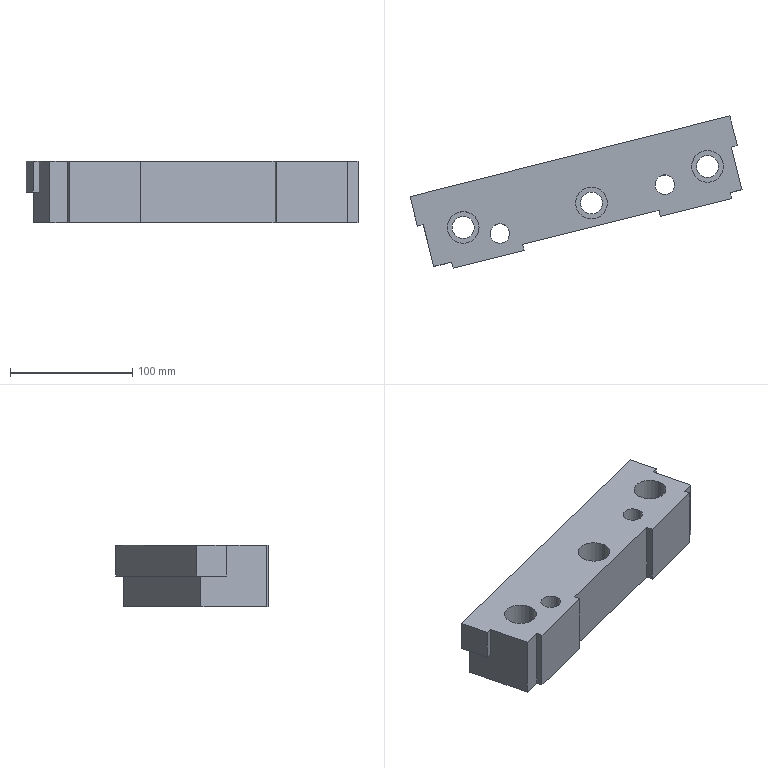Part | NX | features solid 2 | 1 solid | 31 faces | box 271.707 x 124.488 x 50 mm | volume 708876 mm3 | plane 19 | cylinder 8 | spline 4 | commonest cylinder face diameters 18 x3 26 x3 16 x2
STEP:
#1=CARTESIAN_POINT('',(-52.501,508.185,0.));
#2=VERTEX_POINT('',#1);
#3=CARTESIAN_POINT('',(-47.652,509.406,0.));
#4=VERTEX_POINT('',#3);
#5=CARTESIAN_POINT('',(-47.652,509.406,0.));
#6=CARTESIAN_POINT('',(-49.268,508.999,0.));
#7=CARTESIAN_POINT('',(-50.884,508.592,0.));
#8=CARTESIAN_POINT('',(-52.501,508.185,0.));
#9=B_SPLINE_CURVE_WITH_KNOTS('',3,(#5,#6,#7,#8),.UNSPECIFIED.,.F.,.F.,(4,4),(1.091,1.096),.UNSPECIFIED.);
#10=EDGE_CURVE('',#2,#4,#9,.F.);
#11=ORIENTED_EDGE('',*,*,#10,.F.);
#12=CARTESIAN_POINT('',(-52.501,508.185,-25.));
#13=VERTEX_POINT('',#12);
#14=CARTESIAN_POINT('',(-52.501,508.185,-25.));
#15=DIRECTION('',(0.,0.,-1.));
#16=VECTOR('',#15,1000.);
#17=LINE('',#14,#16);
#18=EDGE_CURVE('',#13,#2,#17,.F.);
#19=ORIENTED_EDGE('',*,*,#18,.F.);
#20=CARTESIAN_POINT('',(-47.652,509.406,-25.));
#21=VERTEX_POINT('',#20);
#22=CARTESIAN_POINT('',(-52.501,508.185,-25.));
#23=CARTESIAN_POINT('',(-50.884,508.592,-25.));
#24=CARTESIAN_POINT('',(-49.268,508.999,-25.));
#25=CARTESIAN_POINT('',(-47.652,509.406,-25.));
#26=B_SPLINE_CURVE_WITH_KNOTS('',3,(#22,#23,#24,#25),.UNSPECIFIED.,.F.,.F.,(4,4),(0.9813,0.9998),.UNSPECIFIED.);
#27=EDGE_CURVE('',#13,#21,#26,.T.);
#28=ORIENTED_EDGE('',*,*,#27,.T.);
#29=CARTESIAN_POINT('',(-47.652,509.406,-12.5));
#30=DIRECTION('',(0.,0.,-1.));
#31=VECTOR('',#30,1000.);
#32=LINE('',#29,#31);
#33=EDGE_CURVE('',#21,#4,#32,.F.);
#34=ORIENTED_EDGE('',*,*,#33,.T.);
#35=EDGE_LOOP('',(#11,#19,#28,#34));
#36=FACE_BOUND('',#35,.T.);
#37=CARTESIAN_POINT('',(-52.501,508.185,0.));
#38=CARTESIAN_POINT('',(-52.501,508.185,-25.));
#39=CARTESIAN_POINT('',(-50.884,508.592,0.));
#40=CARTESIAN_POINT('',(-50.884,508.592,-25.));
#41=CARTESIAN_POINT('',(-49.268,508.999,0.));
#42=CARTESIAN_POINT('',(-49.268,508.999,-25.));
#43=CARTESIAN_POINT('',(-47.652,509.406,0.));
#44=CARTESIAN_POINT('',(-47.652,509.406,-25.));
#45=B_SPLINE_SURFACE_WITH_KNOTS('',3,1,((#37,#38),(#39,#40),(#41,#42),(#43,#44)),.SURF_OF_LINEAR_EXTRUSION.,.F.,.F.,.F.,(4,4),(2,2),(0.9813,0.9998),(0.,1.),.PIECEWISE_BEZIER_KNOTS.);
#46=ADVANCED_FACE('',(#36),#45,.F.);
#47=CARTESIAN_POINT('',(-262.995,442.377,-50.));
#48=VERTEX_POINT('',#47);
#49=CARTESIAN_POINT('',(-271.995,442.377,-50.));
#50=DIRECTION('',(0.,0.,1.));
#51=DIRECTION('',(1.,0.,0.));
#52=AXIS2_PLACEMENT_3D('',#49,#50,#51);
#53=CIRCLE('',#52,9.);
#54=EDGE_CURVE('',#48,#48,#53,.T.);
#55=ORIENTED_EDGE('',*,*,#54,.F.);
#56=EDGE_LOOP('',(#55));
#57=FACE_BOUND('',#56,.T.);
#58=CARTESIAN_POINT('',(-262.995,442.377,-30.));
#59=VERTEX_POINT('',#58);
#60=CARTESIAN_POINT('',(-271.995,442.377,-30.));
#61=DIRECTION('',(0.,0.,1.));
#62=DIRECTION('',(1.,0.,0.));
#63=AXIS2_PLACEMENT_3D('',#60,#61,#62);
#64=CIRCLE('',#63,9.);
#65=EDGE_CURVE('',#59,#59,#64,.F.);
#66=ORIENTED_EDGE('',*,*,#65,.F.);
#67=EDGE_LOOP('',(#66));
#68=FACE_BOUND('',#67,.T.);
#69=CARTESIAN_POINT('',(-271.995,442.377,-125.));
#70=DIRECTION('',(0.,0.,1.));
#71=DIRECTION('',(1.,0.,0.));
#72=AXIS2_PLACEMENT_3D('',#69,#70,#71);
#73=CYLINDRICAL_SURFACE('',#72,9.);
#74=ADVANCED_FACE('',(#57,#68),#73,.F.);
#75=CARTESIAN_POINT('',(-157.995,462.377,-50.));
#76=VERTEX_POINT('',#75);
#77=CARTESIAN_POINT('',(-166.995,462.377,-50.));
#78=DIRECTION('',(0.,0.,1.));
#79=DIRECTION('',(1.,0.,0.));
#80=AXIS2_PLACEMENT_3D('',#77,#78,#79);
#81=CIRCLE('',#80,9.);
#82=EDGE_CURVE('',#76,#76,#81,.T.);
#83=ORIENTED_EDGE('',*,*,#82,.F.);
#84=EDGE_LOOP('',(#83));
#85=FACE_BOUND('',#84,.T.);
#86=CARTESIAN_POINT('',(-157.995,462.377,-30.));
#87=VERTEX_POINT('',#86);
#88=CARTESIAN_POINT('',(-166.995,462.377,-30.));
#89=DIRECTION('',(0.,0.,1.));
#90=DIRECTION('',(1.,0.,0.));
#91=AXIS2_PLACEMENT_3D('',#88,#89,#90);
#92=CIRCLE('',#91,9.);
#93=EDGE_CURVE('',#87,#87,#92,.F.);
#94=ORIENTED_EDGE('',*,*,#93,.F.);
#95=EDGE_LOOP('',(#94));
#96=FACE_BOUND('',#95,.T.);
#97=CARTESIAN_POINT('',(-166.995,462.377,-125.));
#98=DIRECTION('',(0.,0.,1.));
#99=DIRECTION('',(1.,0.,0.));
#100=AXIS2_PLACEMENT_3D('',#97,#98,#99);
#101=CYLINDRICAL_SURFACE('',#100,9.);
#102=ADVANCED_FACE('',(#85,#96),#101,.F.);
#103=CARTESIAN_POINT('',(-62.995,492.377,-50.));
#104=VERTEX_POINT('',#103);
#105=CARTESIAN_POINT('',(-71.995,492.377,-50.));
#106=DIRECTION('',(0.,0.,1.));
#107=DIRECTION('',(1.,0.,0.));
#108=AXIS2_PLACEMENT_3D('',#105,#106,#107);
#109=CIRCLE('',#108,9.);
#110=EDGE_CURVE('',#104,#104,#109,.T.);
#111=ORIENTED_EDGE('',*,*,#110,.F.);
#112=EDGE_LOOP('',(#111));
#113=FACE_BOUND('',#112,.T.);
#114=CARTESIAN_POINT('',(-62.995,492.377,-30.));
#115=VERTEX_POINT('',#114);
#116=CARTESIAN_POINT('',(-71.995,492.377,-30.));
#117=DIRECTION('',(0.,0.,1.));
#118=DIRECTION('',(1.,0.,0.));
#119=AXIS2_PLACEMENT_3D('',#116,#117,#118);
#120=CIRCLE('',#119,9.);
#121=EDGE_CURVE('',#115,#115,#120,.F.);
#122=ORIENTED_EDGE('',*,*,#121,.F.);
#123=EDGE_LOOP('',(#122));
#124=FACE_BOUND('',#123,.T.);
#125=CARTESIAN_POINT('',(-71.995,492.377,-125.));
#126=DIRECTION('',(0.,0.,1.));
#127=DIRECTION('',(1.,0.,0.));
#128=AXIS2_PLACEMENT_3D('',#125,#126,#127);
#129=CYLINDRICAL_SURFACE('',#128,9.);
#130=ADVANCED_FACE('',(#113,#124),#129,.F.);
#131=CARTESIAN_POINT('',(-43.802,473.297,0.));
#132=VERTEX_POINT('',#131);
#133=CARTESIAN_POINT('',(-53.505,470.878,0.));
#134=VERTEX_POINT('',#133);
#135=CARTESIAN_POINT('',(-300.93,409.188,0.));
#136=DIRECTION('',(-0.9703,-0.2419,0.));
#137=VECTOR('',#136,1000.);
#138=LINE('',#135,#137);
#139=EDGE_CURVE('',#132,#134,#138,.T.);
#140=ORIENTED_EDGE('',*,*,#139,.T.);
#141=CARTESIAN_POINT('',(-53.505,470.878,-50.));
#142=VERTEX_POINT('',#141);
#143=CARTESIAN_POINT('',(-53.505,470.878,-70.));
#144=DIRECTION('',(0.,0.,-1.));
#145=VECTOR('',#144,1000.);
#146=LINE('',#143,#145);
#147=EDGE_CURVE('',#134,#142,#146,.T.);
#148=ORIENTED_EDGE('',*,*,#147,.T.);
#149=CARTESIAN_POINT('',(-43.802,473.297,-50.));
#150=VERTEX_POINT('',#149);
#151=CARTESIAN_POINT('',(-363.329,393.63,-50.));
#152=DIRECTION('',(0.9703,0.2419,0.));
#153=VECTOR('',#152,1000.);
#154=LINE('',#151,#153);
#155=EDGE_CURVE('',#142,#150,#154,.T.);
#156=ORIENTED_EDGE('',*,*,#155,.T.);
#157=CARTESIAN_POINT('',(-43.802,473.297,-70.));
#158=DIRECTION('',(0.,0.,1.));
#159=VECTOR('',#158,1000.);
#160=LINE('',#157,#159);
#161=EDGE_CURVE('',#150,#132,#160,.T.);
#162=ORIENTED_EDGE('',*,*,#161,.T.);
#163=EDGE_LOOP('',(#140,#148,#156,#162));
#164=FACE_BOUND('',#163,.T.);
#165=CARTESIAN_POINT('',(-300.93,409.188,-70.));
#166=DIRECTION('',(0.2419,-0.9703,0.));
#167=DIRECTION('',(0.9703,0.2419,0.));
#168=AXIS2_PLACEMENT_3D('',#165,#166,#167);
#169=PLANE('',#168);
#170=ADVANCED_FACE('',(#164),#169,.T.);
#171=CARTESIAN_POINT('',(-111.723,456.363,0.));
#172=VERTEX_POINT('',#171);
#173=CARTESIAN_POINT('',(-111.723,456.363,-50.));
#174=VERTEX_POINT('',#173);
#175=CARTESIAN_POINT('',(-111.723,456.363,-70.));
#176=DIRECTION('',(0.,0.,-1.));
#177=VECTOR('',#176,1000.);
#178=LINE('',#175,#177);
#179=EDGE_CURVE('',#172,#174,#178,.T.);
#180=ORIENTED_EDGE('',*,*,#179,.F.);
#181=CARTESIAN_POINT('',(-223.307,428.542,0.));
#182=VERTEX_POINT('',#181);
#183=CARTESIAN_POINT('',(-300.93,409.188,0.));
#184=DIRECTION('',(-0.9703,-0.2419,0.));
#185=VECTOR('',#184,1000.);
#186=LINE('',#183,#185);
#187=EDGE_CURVE('',#172,#182,#186,.T.);
#188=ORIENTED_EDGE('',*,*,#187,.T.);
#189=CARTESIAN_POINT('',(-223.307,428.542,-50.));
#190=VERTEX_POINT('',#189);
#191=CARTESIAN_POINT('',(-223.307,428.542,-70.));
#192=DIRECTION('',(0.,0.,-1.));
#193=VECTOR('',#192,1000.);
#194=LINE('',#191,#193);
#195=EDGE_CURVE('',#182,#190,#194,.T.);
#196=ORIENTED_EDGE('',*,*,#195,.T.);
#197=CARTESIAN_POINT('',(-363.329,393.63,-50.));
#198=DIRECTION('',(0.9703,0.2419,0.));
#199=VECTOR('',#198,1000.);
#200=LINE('',#197,#199);
#201=EDGE_CURVE('',#190,#174,#200,.T.);
#202=ORIENTED_EDGE('',*,*,#201,.T.);
#203=EDGE_LOOP('',(#180,#188,#196,#202));
#204=FACE_BOUND('',#203,.T.);
#205=CARTESIAN_POINT('',(-300.93,409.188,-70.));
#206=DIRECTION('',(0.2419,-0.9703,0.));
#207=DIRECTION('',(0.9703,0.2419,0.));
#208=AXIS2_PLACEMENT_3D('',#205,#206,#207);
#209=PLANE('',#208);
#210=ADVANCED_FACE('',(#204),#209,.T.);
#211=CARTESIAN_POINT('',(-281.525,414.026,0.));
#212=VERTEX_POINT('',#211);
#213=CARTESIAN_POINT('',(-281.525,414.026,-50.));
#214=VERTEX_POINT('',#213);
#215=CARTESIAN_POINT('',(-281.525,414.026,-70.));
#216=DIRECTION('',(0.,0.,-1.));
#217=VECTOR('',#216,1000.);
#218=LINE('',#215,#217);
#219=EDGE_CURVE('',#212,#214,#218,.T.);
#220=ORIENTED_EDGE('',*,*,#219,.F.);
#221=CARTESIAN_POINT('',(-296.079,410.398,0.));
#222=VERTEX_POINT('',#221);
#223=CARTESIAN_POINT('',(-300.93,409.188,0.));
#224=DIRECTION('',(-0.9703,-0.2419,0.));
#225=VECTOR('',#224,1000.);
#226=LINE('',#223,#225);
#227=EDGE_CURVE('',#212,#222,#226,.T.);
#228=ORIENTED_EDGE('',*,*,#227,.T.);
#229=CARTESIAN_POINT('',(-296.079,410.398,-50.));
#230=VERTEX_POINT('',#229);
#231=CARTESIAN_POINT('',(-296.079,410.398,-70.));
#232=DIRECTION('',(0.,0.,1.));
#233=VECTOR('',#232,1000.);
#234=LINE('',#231,#233);
#235=EDGE_CURVE('',#230,#222,#234,.T.);
#236=ORIENTED_EDGE('',*,*,#235,.F.);
#237=CARTESIAN_POINT('',(-363.329,393.63,-50.));
#238=DIRECTION('',(0.9703,0.2419,0.));
#239=VECTOR('',#238,1000.);
#240=LINE('',#237,#239);
#241=EDGE_CURVE('',#230,#214,#240,.T.);
#242=ORIENTED_EDGE('',*,*,#241,.T.);
#243=EDGE_LOOP('',(#220,#228,#236,#242));
#244=FACE_BOUND('',#243,.T.);
#245=CARTESIAN_POINT('',(-300.93,409.188,-70.));
#246=DIRECTION('',(0.2419,-0.9703,0.));
#247=DIRECTION('',(0.9703,0.2419,0.));
#248=AXIS2_PLACEMENT_3D('',#245,#246,#247);
#249=PLANE('',#248);
#250=ADVANCED_FACE('',(#244),#249,.T.);
#251=CARTESIAN_POINT('',(-309.461,443.4,0.));
#252=VERTEX_POINT('',#251);
#253=CARTESIAN_POINT('',(-315.509,467.66,0.));
#254=VERTEX_POINT('',#253);
#255=CARTESIAN_POINT('',(14.033,-854.063,0.));
#256=DIRECTION('',(-0.2419,0.9703,0.));
#257=VECTOR('',#256,1000.);
#258=LINE('',#255,#257);
#259=EDGE_CURVE('',#252,#254,#258,.T.);
#260=ORIENTED_EDGE('',*,*,#259,.F.);
#261=CARTESIAN_POINT('',(-304.623,444.665,0.));
#262=VERTEX_POINT('',#261);
#263=CARTESIAN_POINT('',(-304.623,444.665,0.));
#264=CARTESIAN_POINT('',(-306.236,444.246,0.));
#265=CARTESIAN_POINT('',(-307.849,443.824,0.));
#266=CARTESIAN_POINT('',(-309.461,443.4,0.));
#267=B_SPLINE_CURVE_WITH_KNOTS('',3,(#263,#264,#265,#266),.UNSPECIFIED.,.F.,.F.,(4,4),(1.356,1.361),.UNSPECIFIED.);
#268=EDGE_CURVE('',#252,#262,#267,.F.);
#269=ORIENTED_EDGE('',*,*,#268,.T.);
#270=CARTESIAN_POINT('',(-285.193,366.734,0.));
#271=DIRECTION('',(0.2419,-0.9703,0.));
#272=VECTOR('',#271,1000.);
#273=LINE('',#270,#272);
#274=EDGE_CURVE('',#262,#222,#273,.T.);
#275=ORIENTED_EDGE('',*,*,#274,.T.);
#276=ORIENTED_EDGE('',*,*,#227,.F.);
#277=CARTESIAN_POINT('',(-280.315,409.175,0.));
#278=VERTEX_POINT('',#277);
#279=CARTESIAN_POINT('',(-296.103,472.498,0.));
#280=DIRECTION('',(0.2419,-0.9703,0.));
#281=VECTOR('',#280,1000.);
#282=LINE('',#279,#281);
#283=EDGE_CURVE('',#212,#278,#282,.T.);
#284=ORIENTED_EDGE('',*,*,#283,.T.);
#285=CARTESIAN_POINT('',(-222.097,423.69,0.));
#286=VERTEX_POINT('',#285);
#287=CARTESIAN_POINT('',(-362.119,388.779,0.));
#288=DIRECTION('',(0.9703,0.2419,0.));
#289=VECTOR('',#288,1000.);
#290=LINE('',#287,#289);
#291=EDGE_CURVE('',#278,#286,#290,.T.);
#292=ORIENTED_EDGE('',*,*,#291,.T.);
#293=CARTESIAN_POINT('',(-237.885,487.014,0.));
#294=DIRECTION('',(0.2419,-0.9703,0.));
#295=VECTOR('',#294,1000.);
#296=LINE('',#293,#295);
#297=EDGE_CURVE('',#182,#286,#296,.T.);
#298=ORIENTED_EDGE('',*,*,#297,.F.);
#299=ORIENTED_EDGE('',*,*,#187,.F.);
#300=CARTESIAN_POINT('',(-110.513,451.511,0.));
#301=VERTEX_POINT('',#300);
#302=CARTESIAN_POINT('',(-126.301,514.835,0.));
#303=DIRECTION('',(0.2419,-0.9703,0.));
#304=VECTOR('',#303,1000.);
#305=LINE('',#302,#304);
#306=EDGE_CURVE('',#172,#301,#305,.T.);
#307=ORIENTED_EDGE('',*,*,#306,.T.);
#308=CARTESIAN_POINT('',(-52.295,466.027,0.));
#309=VERTEX_POINT('',#308);
#310=CARTESIAN_POINT('',(-362.119,388.779,0.));
#311=DIRECTION('',(0.9703,0.2419,0.));
#312=VECTOR('',#311,1000.);
#313=LINE('',#310,#312);
#314=EDGE_CURVE('',#301,#309,#313,.T.);
#315=ORIENTED_EDGE('',*,*,#314,.T.);
#316=CARTESIAN_POINT('',(-68.084,529.35,0.));
#317=DIRECTION('',(0.2419,-0.9703,0.));
#318=VECTOR('',#317,1000.);
#319=LINE('',#316,#318);
#320=EDGE_CURVE('',#134,#309,#319,.T.);
#321=ORIENTED_EDGE('',*,*,#320,.F.);
#322=ORIENTED_EDGE('',*,*,#139,.F.);
#323=CARTESIAN_POINT('',(-32.916,429.634,0.));
#324=DIRECTION('',(0.2419,-0.9703,0.));
#325=VECTOR('',#324,1000.);
#326=LINE('',#323,#325);
#327=EDGE_CURVE('',#2,#132,#326,.T.);
#328=ORIENTED_EDGE('',*,*,#327,.F.);
#329=ORIENTED_EDGE('',*,*,#10,.T.);
#330=CARTESIAN_POINT('',(-53.7,533.663,0.));
#331=VERTEX_POINT('',#330);
#332=CARTESIAN_POINT('',(276.013,-788.744,0.));
#333=DIRECTION('',(-0.2419,0.9703,0.));
#334=VECTOR('',#333,1000.);
#335=LINE('',#332,#334);
#336=EDGE_CURVE('',#4,#331,#335,.T.);
#337=ORIENTED_EDGE('',*,*,#336,.T.);
#338=CARTESIAN_POINT('',(-53.7,533.663,0.));
#339=CARTESIAN_POINT('',(-75.519,528.17,0.));
#340=CARTESIAN_POINT('',(-119.156,517.175,0.));
#341=CARTESIAN_POINT('',(-184.597,500.638,0.));
#342=CARTESIAN_POINT('',(-239.173,486.991,0.));
#343=CARTESIAN_POINT('',(-282.82,476.03,0.));
#344=CARTESIAN_POINT('',(-304.634,470.521,0.));
#345=CARTESIAN_POINT('',(-315.509,467.66,0.));
#346=B_SPLINE_CURVE_WITH_KNOTS('',3,(#338,#339,#340,#341,#342,#343,#344,#345),.UNSPECIFIED.,.F.,.F.,(4,1,1,1,1,4),(2.049,2.116,2.184,2.251,2.285,2.319),.UNSPECIFIED.);
#347=EDGE_CURVE('',#254,#331,#346,.F.);
#348=ORIENTED_EDGE('',*,*,#347,.F.);
#349=EDGE_LOOP('',(#260,#269,#275,#276,#284,#292,#298,#299,#307,#315,#321,#322,#328,#329,#337,#348));
#350=FACE_BOUND('',#349,.T.);
#351=CARTESIAN_POINT('',(-258.995,442.377,0.));
#352=VERTEX_POINT('',#351);
#353=CARTESIAN_POINT('',(-271.995,442.377,0.));
#354=DIRECTION('',(0.,0.,1.));
#355=DIRECTION('',(1.,0.,0.));
#356=AXIS2_PLACEMENT_3D('',#353,#354,#355);
#357=CIRCLE('',#356,13.);
#358=EDGE_CURVE('',#352,#352,#357,.T.);
#359=ORIENTED_EDGE('',*,*,#358,.F.);
#360=EDGE_LOOP('',(#359));
#361=FACE_BOUND('',#360,.T.);
#362=CARTESIAN_POINT('',(-153.995,462.377,0.));
#363=VERTEX_POINT('',#362);
#364=CARTESIAN_POINT('',(-166.995,462.377,0.));
#365=DIRECTION('',(0.,0.,1.));
#366=DIRECTION('',(1.,0.,0.));
#367=AXIS2_PLACEMENT_3D('',#364,#365,#366);
#368=CIRCLE('',#367,13.);
#369=EDGE_CURVE('',#363,#363,#368,.T.);
#370=ORIENTED_EDGE('',*,*,#369,.F.);
#371=EDGE_LOOP('',(#370));
#372=FACE_BOUND('',#371,.T.);
#373=CARTESIAN_POINT('',(-58.995,492.377,0.));
#374=VERTEX_POINT('',#373);
#375=CARTESIAN_POINT('',(-71.995,492.377,0.));
#376=DIRECTION('',(0.,0.,1.));
#377=DIRECTION('',(1.,0.,0.));
#378=AXIS2_PLACEMENT_3D('',#375,#376,#377);
#379=CIRCLE('',#378,13.);
#380=EDGE_CURVE('',#374,#374,#379,.T.);
#381=ORIENTED_EDGE('',*,*,#380,.F.);
#382=EDGE_LOOP('',(#381));
#383=FACE_BOUND('',#382,.T.);
#384=CARTESIAN_POINT('',(-233.995,437.377,0.));
#385=VERTEX_POINT('',#384);
#386=CARTESIAN_POINT('',(-241.995,437.377,0.));
#387=DIRECTION('',(0.,0.,1.));
#388=DIRECTION('',(1.,0.,0.));
#389=AXIS2_PLACEMENT_3D('',#386,#387,#388);
#390=CIRCLE('',#389,8.);
#391=EDGE_CURVE('',#385,#385,#390,.T.);
#392=ORIENTED_EDGE('',*,*,#391,.F.);
#393=EDGE_LOOP('',(#392));
#394=FACE_BOUND('',#393,.T.);
#395=CARTESIAN_POINT('',(-98.995,477.377,0.));
#396=VERTEX_POINT('',#395);
#397=CARTESIAN_POINT('',(-106.995,477.377,0.));
#398=DIRECTION('',(0.,0.,1.));
#399=DIRECTION('',(1.,0.,0.));
#400=AXIS2_PLACEMENT_3D('',#397,#398,#399);
#401=CIRCLE('',#400,8.);
#402=EDGE_CURVE('',#396,#396,#401,.T.);
#403=ORIENTED_EDGE('',*,*,#402,.F.);
#404=EDGE_LOOP('',(#403));
#405=FACE_BOUND('',#404,.T.);
#406=CARTESIAN_POINT('',(-48.365,-869.621,0.));
#407=DIRECTION('',(0.,0.,1.));
#408=DIRECTION('',(1.,0.,0.));
#409=AXIS2_PLACEMENT_3D('',#406,#407,#408);
#410=PLANE('',#409);
#411=ADVANCED_FACE('',(#350,#361,#372,#383,#394,#405),#410,.T.);
#412=CARTESIAN_POINT('',(-309.461,443.4,-25.));
#413=VERTEX_POINT('',#412);
#414=CARTESIAN_POINT('',(-304.623,444.665,-25.));
#415=VERTEX_POINT('',#414);
#416=CARTESIAN_POINT('',(-309.461,443.4,-25.));
#417=CARTESIAN_POINT('',(-307.824,443.831,-25.));
#418=CARTESIAN_POINT('',(-306.238,444.246,-25.));
#419=CARTESIAN_POINT('',(-304.623,444.665,-25.));
#420=B_SPLINE_CURVE_WITH_KNOTS('',3,(#416,#417,#418,#419),.UNSPECIFIED.,.F.,.F.,(4,4),(-0.001195,0.01761),.UNSPECIFIED.);
#421=EDGE_CURVE('',#413,#415,#420,.T.);
#422=ORIENTED_EDGE('',*,*,#421,.F.);
#423=CARTESIAN_POINT('',(-315.509,467.66,-25.));
#424=VERTEX_POINT('',#423);
#425=CARTESIAN_POINT('',(-315.509,467.66,-25.));
#426=DIRECTION('',(0.2419,-0.9703,0.));
#427=VECTOR('',#426,1000.);
#428=LINE('',#425,#427);
#429=EDGE_CURVE('',#424,#413,#428,.T.);
#430=ORIENTED_EDGE('',*,*,#429,.F.);
#431=CARTESIAN_POINT('',(-53.7,533.663,-25.));
#432=VERTEX_POINT('',#431);
#433=CARTESIAN_POINT('',(-315.509,467.66,-25.));
#434=CARTESIAN_POINT('',(-304.633,470.521,-25.));
#435=CARTESIAN_POINT('',(-282.818,476.031,-25.));
#436=CARTESIAN_POINT('',(-239.172,486.991,-25.));
#437=CARTESIAN_POINT('',(-184.599,500.638,-25.));
#438=CARTESIAN_POINT('',(-119.156,517.175,-25.));
#439=CARTESIAN_POINT('',(-75.519,528.17,-25.));
#440=CARTESIAN_POINT('',(-53.7,533.663,-25.));
#441=B_SPLINE_CURVE_WITH_KNOTS('',3,(#433,#434,#435,#436,#437,#438,#439,#440),.UNSPECIFIED.,.F.,.F.,(4,1,1,1,1,4),(0.4881,0.5217,0.5553,0.6226,0.6898,0.757),.UNSPECIFIED.);
#442=EDGE_CURVE('',#424,#432,#441,.T.);
#443=ORIENTED_EDGE('',*,*,#442,.T.);
#444=CARTESIAN_POINT('',(558.557,-1921.963,-25.));
#445=DIRECTION('',(-0.2419,0.9703,0.));
#446=VECTOR('',#445,1000.);
#447=LINE('',#444,#446);
#448=EDGE_CURVE('',#21,#432,#447,.T.);
#449=ORIENTED_EDGE('',*,*,#448,.F.);
#450=ORIENTED_EDGE('',*,*,#27,.F.);
#451=CARTESIAN_POINT('',(-57.339,527.591,-25.));
#452=VERTEX_POINT('',#451);
#453=CARTESIAN_POINT('',(-32.916,429.634,-25.));
#454=DIRECTION('',(-0.2419,0.9703,0.));
#455=VECTOR('',#454,1000.);
#456=LINE('',#453,#455);
#457=EDGE_CURVE('',#13,#452,#456,.T.);
#458=ORIENTED_EDGE('',*,*,#457,.T.);
#459=CARTESIAN_POINT('',(-309.462,464.072,-25.));
#460=VERTEX_POINT('',#459);
#461=CARTESIAN_POINT('',(-57.339,527.591,-25.));
#462=CARTESIAN_POINT('',(-78.35,522.301,-25.));
#463=CARTESIAN_POINT('',(-120.369,511.708,-25.));
#464=CARTESIAN_POINT('',(-183.392,495.797,-25.));
#465=CARTESIAN_POINT('',(-246.439,479.985,-25.));
#466=CARTESIAN_POINT('',(-288.49,469.519,-25.));
#467=CARTESIAN_POINT('',(-309.462,464.072,-25.));
#468=B_SPLINE_CURVE_WITH_KNOTS('',3,(#461,#462,#463,#464,#465,#466,#467),.UNSPECIFIED.,.F.,.F.,(4,1,1,1,4),(1.096,1.161,1.226,1.291,1.356),.UNSPECIFIED.);
#469=EDGE_CURVE('',#460,#452,#468,.F.);
#470=ORIENTED_EDGE('',*,*,#469,.F.);
#471=CARTESIAN_POINT('',(-285.193,366.734,-25.));
#472=DIRECTION('',(-0.2419,0.9703,0.));
#473=VECTOR('',#472,1000.);
#474=LINE('',#471,#473);
#475=EDGE_CURVE('',#415,#460,#474,.T.);
#476=ORIENTED_EDGE('',*,*,#475,.F.);
#477=EDGE_LOOP('',(#422,#430,#443,#449,#450,#458,#470,#476));
#478=FACE_BOUND('',#477,.T.);
#479=CARTESIAN_POINT('',(-315.509,467.66,-25.));
#480=DIRECTION('',(0.,0.,-1.));
#481=DIRECTION('',(-1.,0.,0.));
#482=AXIS2_PLACEMENT_3D('',#479,#480,#481);
#483=PLANE('',#482);
#484=ADVANCED_FACE('',(#478),#483,.T.);
#485=ORIENTED_EDGE('',*,*,#457,.F.);
#486=ORIENTED_EDGE('',*,*,#18,.T.);
#487=ORIENTED_EDGE('',*,*,#327,.T.);
#488=ORIENTED_EDGE('',*,*,#161,.F.);
#489=CARTESIAN_POINT('',(-57.339,527.591,-50.));
#490=VERTEX_POINT('',#489);
#491=CARTESIAN_POINT('',(271.162,-789.954,-50.));
#492=DIRECTION('',(-0.2419,0.9703,0.));
#493=VECTOR('',#492,1000.);
#494=LINE('',#491,#493);
#495=EDGE_CURVE('',#150,#490,#494,.T.);
#496=ORIENTED_EDGE('',*,*,#495,.T.);
#497=CARTESIAN_POINT('',(-57.339,527.591,-42.5));
#498=DIRECTION('',(0.,0.,1.));
#499=VECTOR('',#498,1000.);
#500=LINE('',#497,#499);
#501=EDGE_CURVE('',#490,#452,#500,.T.);
#502=ORIENTED_EDGE('',*,*,#501,.T.);
#503=EDGE_LOOP('',(#485,#486,#487,#488,#496,#502));
#504=FACE_BOUND('',#503,.T.);
#505=CARTESIAN_POINT('',(-32.916,429.634,-70.));
#506=DIRECTION('',(0.9703,0.2419,0.));
#507=DIRECTION('',(-0.2419,0.9703,0.));
#508=AXIS2_PLACEMENT_3D('',#505,#506,#507);
#509=PLANE('',#508);
#510=ADVANCED_FACE('',(#504),#509,.T.);
#511=ORIENTED_EDGE('',*,*,#274,.F.);
#512=CARTESIAN_POINT('',(-304.623,444.665,-25.));
#513=DIRECTION('',(0.,0.,-1.));
#514=VECTOR('',#513,1000.);
#515=LINE('',#512,#514);
#516=EDGE_CURVE('',#415,#262,#515,.F.);
#517=ORIENTED_EDGE('',*,*,#516,.F.);
#518=ORIENTED_EDGE('',*,*,#475,.T.);
#519=CARTESIAN_POINT('',(-309.462,464.072,-50.));
#520=VERTEX_POINT('',#519);
#521=CARTESIAN_POINT('',(-309.462,464.072,-42.5));
#522=DIRECTION('',(0.,0.,1.));
#523=VECTOR('',#522,1000.);
#524=LINE('',#521,#523);
#525=EDGE_CURVE('',#520,#460,#524,.T.);
#526=ORIENTED_EDGE('',*,*,#525,.F.);
#527=CARTESIAN_POINT('',(18.885,-852.853,-50.));
#528=DIRECTION('',(-0.2419,0.9703,0.));
#529=VECTOR('',#528,1000.);
#530=LINE('',#527,#529);
#531=EDGE_CURVE('',#230,#520,#530,.T.);
#532=ORIENTED_EDGE('',*,*,#531,.F.);
#533=ORIENTED_EDGE('',*,*,#235,.T.);
#534=EDGE_LOOP('',(#511,#517,#518,#526,#532,#533));
#535=FACE_BOUND('',#534,.T.);
#536=CARTESIAN_POINT('',(-285.193,366.734,-70.));
#537=DIRECTION('',(0.9703,0.2419,0.));
#538=DIRECTION('',(-0.2419,0.9703,0.));
#539=AXIS2_PLACEMENT_3D('',#536,#537,#538);
#540=PLANE('',#539);
#541=ADVANCED_FACE('',(#535),#540,.F.);
#542=ORIENTED_EDGE('',*,*,#54,.T.);
#543=EDGE_LOOP('',(#542));
#544=FACE_BOUND('',#543,.T.);
#545=CARTESIAN_POINT('',(-233.995,437.377,-50.));
#546=VERTEX_POINT('',#545);
#547=CARTESIAN_POINT('',(-241.995,437.377,-50.));
#548=DIRECTION('',(0.,0.,1.));
#549=DIRECTION('',(1.,0.,0.));
#550=AXIS2_PLACEMENT_3D('',#547,#548,#549);
#551=CIRCLE('',#550,8.);
#552=EDGE_CURVE('',#546,#546,#551,.T.);
#553=ORIENTED_EDGE('',*,*,#552,.T.);
#554=EDGE_LOOP('',(#553));
#555=FACE_BOUND('',#554,.T.);
#556=ORIENTED_EDGE('',*,*,#82,.T.);
#557=EDGE_LOOP('',(#556));
#558=FACE_BOUND('',#557,.T.);
#559=CARTESIAN_POINT('',(-98.995,477.377,-50.));
#560=VERTEX_POINT('',#559);
#561=CARTESIAN_POINT('',(-106.995,477.377,-50.));
#562=DIRECTION('',(0.,0.,1.));
#563=DIRECTION('',(1.,0.,0.));
#564=AXIS2_PLACEMENT_3D('',#561,#562,#563);
#565=CIRCLE('',#564,8.);
#566=EDGE_CURVE('',#560,#560,#565,.T.);
#567=ORIENTED_EDGE('',*,*,#566,.T.);
#568=EDGE_LOOP('',(#567));
#569=FACE_BOUND('',#568,.T.);
#570=ORIENTED_EDGE('',*,*,#110,.T.);
#571=EDGE_LOOP('',(#570));
#572=FACE_BOUND('',#571,.T.);
#573=ORIENTED_EDGE('',*,*,#531,.T.);
#574=CARTESIAN_POINT('',(-309.462,464.072,-50.));
#575=CARTESIAN_POINT('',(-306.559,464.826,-50.));
#576=CARTESIAN_POINT('',(-301.325,466.172,-50.));
#577=CARTESIAN_POINT('',(-292.584,468.397,-50.));
#578=CARTESIAN_POINT('',(-285.148,470.281,-50.));
#579=CARTESIAN_POINT('',(-276.83,472.38,-50.));
#580=CARTESIAN_POINT('',(-269.164,474.308,-50.));
#581=CARTESIAN_POINT('',(-262.592,475.958,-50.));
#582=CARTESIAN_POINT('',(-257.439,477.251,-50.));
#583=CARTESIAN_POINT('',(-252.972,478.37,-50.));
#584=CARTESIAN_POINT('',(-249.729,479.182,-50.));
#585=CARTESIAN_POINT('',(-247.88,479.645,-50.));
#586=CARTESIAN_POINT('',(-246.389,480.018,-50.));
#587=CARTESIAN_POINT('',(-245.229,480.308,-50.));
#588=CARTESIAN_POINT('',(-243.58,480.72,-50.));
#589=CARTESIAN_POINT('',(-240.775,481.422,-50.));
#590=CARTESIAN_POINT('',(-236.816,482.413,-50.));
#591=CARTESIAN_POINT('',(-232.2,483.568,-50.));
#592=CARTESIAN_POINT('',(-226.206,485.069,-50.));
#593=CARTESIAN_POINT('',(-219.023,486.869,-50.));
#594=CARTESIAN_POINT('',(-210.895,488.906,-50.));
#595=CARTESIAN_POINT('',(-203.261,490.821,-50.));
#596=CARTESIAN_POINT('',(-197.309,492.315,-50.));
#597=CARTESIAN_POINT('',(-192.795,493.449,-50.));
#598=CARTESIAN_POINT('',(-189.529,494.27,-50.));
#599=CARTESIAN_POINT('',(-186.922,494.926,-50.));
#600=CARTESIAN_POINT('',(-185.128,495.377,-50.));
#601=CARTESIAN_POINT('',(-184.154,495.623,-50.));
#602=CARTESIAN_POINT('',(-183.332,495.829,-50.));
#603=CARTESIAN_POINT('',(-182.894,495.94,-50.));
#604=CARTESIAN_POINT('',(-182.151,496.127,-50.));
#605=CARTESIAN_POINT('',(-180.865,496.451,-50.));
#606=CARTESIAN_POINT('',(-178.846,496.959,-50.));
#607=CARTESIAN_POINT('',(-176.203,497.625,-50.));
#608=CARTESIAN_POINT('',(-172.36,498.593,-50.));
#609=CARTESIAN_POINT('',(-166.971,499.951,-50.));
#610=CARTESIAN_POINT('',(-159.563,501.819,-50.));
#611=CARTESIAN_POINT('',(-151.214,503.924,-50.));
#612=CARTESIAN_POINT('',(-143.473,505.876,-50.));
#613=CARTESIAN_POINT('',(-136.81,507.557,-50.));
#614=CARTESIAN_POINT('',(-132.449,508.657,-50.));
#615=CARTESIAN_POINT('',(-128.844,509.566,-50.));
#616=CARTESIAN_POINT('',(-126.078,510.264,-50.));
#617=CARTESIAN_POINT('',(-123.735,510.855,-50.));
#618=CARTESIAN_POINT('',(-122.048,511.281,-50.));
#619=CARTESIAN_POINT('',(-121.11,511.517,-50.));
#620=CARTESIAN_POINT('',(-120.31,511.719,-50.));
#621=CARTESIAN_POINT('',(-119.859,511.833,-50.));
#622=CARTESIAN_POINT('',(-119.138,512.015,-50.));
#623=CARTESIAN_POINT('',(-117.934,512.319,-50.));
#624=CARTESIAN_POINT('',(-116.189,512.759,-50.));
#625=CARTESIAN_POINT('',(-114.115,513.282,-50.));
#626=CARTESIAN_POINT('',(-111.357,513.978,-50.));
#627=CARTESIAN_POINT('',(-107.93,514.842,-50.));
#628=CARTESIAN_POINT('',(-102.488,516.214,-50.));
#629=CARTESIAN_POINT('',(-95.764,517.909,-50.));
#630=CARTESIAN_POINT('',(-87.823,519.911,-50.));
#631=CARTESIAN_POINT('',(-80.007,521.881,-50.));
#632=CARTESIAN_POINT('',(-69.755,524.464,-50.));
#633=CARTESIAN_POINT('',(-62.255,526.353,-50.));
#634=CARTESIAN_POINT('',(-57.339,527.591,-50.));
#635=B_SPLINE_CURVE_WITH_KNOTS('',3,(#574,#575,#576,#577,#578,#579,#580,#581,#582,#583,#584,#585,#586,#587,#588,#589,#590,#591,#592,#593,#594,#595,#596,#597,#598,#599,#600,#601,#602,#603,#604,#605,#606,#607,#608,#609,#610,#611,#612,#613,#614,#615,#616,#617,#618,#619,#620,#621,#622,#623,#624,#625,#626,#627,#628,#629,#630,#631,#632,#633,#634),.UNSPECIFIED.,.F.,.F.,(4,1,1,1,1,1,1,1,1,1,1,1,1,1,1,1,1,1,1,1,1,1,1,1,1,1,1,1,1,1,1,1,1,1,1,1,1,1,1,1,1,1,1,1,1,1,1,1,1,1,1,1,1,1,1,1,1,1,4),(0.,0.0625,0.09375,0.125,0.1562,0.1875,0.2031,0.2188,0.2344,0.2422,0.2461,0.25,0.2539,0.2578,0.2656,0.2812,0.2969,0.3125,0.3438,0.375,0.4062,0.4375,0.4531,0.4688,0.4844,0.4922,0.4961,0.5,0.5039,0.5078,0.5156,0.5312,0.5469,0.5625,0.5938,0.625,0.6562,0.6875,0.7031,0.7188,0.7266,0.7344,0.7422,0.7461,0.748,0.75,0.752,0.7539,0.7578,0.7656,0.7734,0.7812,0.7969,0.8125,0.8438,0.875,0.9062,0.9375,1.),.UNSPECIFIED.);
#636=EDGE_CURVE('',#520,#490,#635,.T.);
#637=ORIENTED_EDGE('',*,*,#636,.T.);
#638=ORIENTED_EDGE('',*,*,#495,.F.);
#639=ORIENTED_EDGE('',*,*,#155,.F.);
#640=CARTESIAN_POINT('',(-52.295,466.027,-50.));
#641=VERTEX_POINT('',#640);
#642=CARTESIAN_POINT('',(-48.667,451.472,-50.));
#643=DIRECTION('',(0.2419,-0.9703,0.));
#644=VECTOR('',#643,1000.);
#645=LINE('',#642,#644);
#646=EDGE_CURVE('',#142,#641,#645,.T.);
#647=ORIENTED_EDGE('',*,*,#646,.T.);
#648=CARTESIAN_POINT('',(-110.513,451.511,-50.));
#649=VERTEX_POINT('',#648);
#650=CARTESIAN_POINT('',(-362.119,388.779,-50.));
#651=DIRECTION('',(0.9703,0.2419,0.));
#652=VECTOR('',#651,1000.);
#653=LINE('',#650,#652);
#654=EDGE_CURVE('',#649,#641,#653,.T.);
#655=ORIENTED_EDGE('',*,*,#654,.F.);
#656=CARTESIAN_POINT('',(-106.884,436.957,-50.));
#657=DIRECTION('',(0.2419,-0.9703,0.));
#658=VECTOR('',#657,1000.);
#659=LINE('',#656,#658);
#660=EDGE_CURVE('',#174,#649,#659,.T.);
#661=ORIENTED_EDGE('',*,*,#660,.F.);
#662=ORIENTED_EDGE('',*,*,#201,.F.);
#663=CARTESIAN_POINT('',(-222.097,423.69,-50.));
#664=VERTEX_POINT('',#663);
#665=CARTESIAN_POINT('',(-218.468,409.136,-50.));
#666=DIRECTION('',(0.2419,-0.9703,0.));
#667=VECTOR('',#666,1000.);
#668=LINE('',#665,#667);
#669=EDGE_CURVE('',#190,#664,#668,.T.);
#670=ORIENTED_EDGE('',*,*,#669,.T.);
#671=CARTESIAN_POINT('',(-280.315,409.175,-50.));
#672=VERTEX_POINT('',#671);
#673=CARTESIAN_POINT('',(-362.119,388.779,-50.));
#674=DIRECTION('',(0.9703,0.2419,0.));
#675=VECTOR('',#674,1000.);
#676=LINE('',#673,#675);
#677=EDGE_CURVE('',#672,#664,#676,.T.);
#678=ORIENTED_EDGE('',*,*,#677,.F.);
#679=CARTESIAN_POINT('',(-276.686,394.621,-50.));
#680=DIRECTION('',(0.2419,-0.9703,0.));
#681=VECTOR('',#680,1000.);
#682=LINE('',#679,#681);
#683=EDGE_CURVE('',#214,#672,#682,.T.);
#684=ORIENTED_EDGE('',*,*,#683,.F.);
#685=ORIENTED_EDGE('',*,*,#241,.F.);
#686=EDGE_LOOP('',(#573,#637,#638,#639,#647,#655,#661,#662,#670,#678,#684,#685));
#687=FACE_BOUND('',#686,.T.);
#688=CARTESIAN_POINT('',(-48.365,-869.621,-50.));
#689=DIRECTION('',(0.,0.,1.));
#690=DIRECTION('',(1.,0.,0.));
#691=AXIS2_PLACEMENT_3D('',#688,#689,#690);
#692=PLANE('',#691);
#693=ADVANCED_FACE('',(#544,#555,#558,#569,#572,#687),#692,.F.);
#694=ORIENTED_EDGE('',*,*,#429,.T.);
#695=CARTESIAN_POINT('',(-309.461,443.4,-12.5));
#696=DIRECTION('',(0.,0.,-1.));
#697=VECTOR('',#696,1000.);
#698=LINE('',#695,#697);
#699=EDGE_CURVE('',#413,#252,#698,.F.);
#700=ORIENTED_EDGE('',*,*,#699,.T.);
#701=ORIENTED_EDGE('',*,*,#259,.T.);
#702=CARTESIAN_POINT('',(-315.509,467.66,-70.));
#703=DIRECTION('',(0.,0.,1.));
#704=VECTOR('',#703,1000.);
#705=LINE('',#702,#704);
#706=EDGE_CURVE('',#424,#254,#705,.T.);
#707=ORIENTED_EDGE('',*,*,#706,.F.);
#708=EDGE_LOOP('',(#694,#700,#701,#707));
#709=FACE_BOUND('',#708,.T.);
#710=CARTESIAN_POINT('',(296.577,-1987.282,-70.));
#711=DIRECTION('',(0.9703,0.2419,0.));
#712=DIRECTION('',(-0.2419,0.9703,0.));
#713=AXIS2_PLACEMENT_3D('',#710,#711,#712);
#714=PLANE('',#713);
#715=ADVANCED_FACE('',(#709),#714,.F.);
#716=ORIENTED_EDGE('',*,*,#636,.F.);
#717=ORIENTED_EDGE('',*,*,#525,.T.);
#718=ORIENTED_EDGE('',*,*,#469,.T.);
#719=ORIENTED_EDGE('',*,*,#501,.F.);
#720=EDGE_LOOP('',(#716,#717,#718,#719));
#721=FACE_BOUND('',#720,.T.);
#722=CARTESIAN_POINT('',(-309.462,464.072,-50.));
#723=CARTESIAN_POINT('',(-309.462,464.072,-25.));
#724=CARTESIAN_POINT('',(-288.545,469.505,-50.));
#725=CARTESIAN_POINT('',(-288.545,469.505,-25.));
#726=CARTESIAN_POINT('',(-246.469,479.978,-50.));
#727=CARTESIAN_POINT('',(-246.469,479.978,-25.));
#728=CARTESIAN_POINT('',(-183.41,495.792,-50.));
#729=CARTESIAN_POINT('',(-183.41,495.792,-25.));
#730=CARTESIAN_POINT('',(-120.374,511.707,-50.));
#731=CARTESIAN_POINT('',(-120.374,511.707,-25.));
#732=CARTESIAN_POINT('',(-78.352,522.3,-50.));
#733=CARTESIAN_POINT('',(-78.352,522.3,-25.));
#734=CARTESIAN_POINT('',(-57.339,527.591,-50.));
#735=CARTESIAN_POINT('',(-57.339,527.591,-25.));
#736=B_SPLINE_SURFACE_WITH_KNOTS('',3,1,((#722,#723),(#724,#725),(#726,#727),(#728,#729),(#730,#731),(#732,#733),(#734,#735)),.SURF_OF_LINEAR_EXTRUSION.,.F.,.F.,.F.,(4,1,1,1,4),(2,2),(0.01834,0.2591,0.4999,0.7407,0.9814),(0.,1.),.UNSPECIFIED.);
#737=ADVANCED_FACE('',(#721),#736,.F.);
#738=ORIENTED_EDGE('',*,*,#442,.F.);
#739=ORIENTED_EDGE('',*,*,#706,.T.);
#740=ORIENTED_EDGE('',*,*,#347,.T.);
#741=CARTESIAN_POINT('',(-53.7,533.663,-70.));
#742=DIRECTION('',(0.,0.,1.));
#743=VECTOR('',#742,1000.);
#744=LINE('',#741,#743);
#745=EDGE_CURVE('',#432,#331,#744,.T.);
#746=ORIENTED_EDGE('',*,*,#745,.F.);
#747=EDGE_LOOP('',(#738,#739,#740,#746));
#748=FACE_BOUND('',#747,.T.);
#749=CARTESIAN_POINT('',(-315.509,467.66,-25.));
#750=CARTESIAN_POINT('',(-315.509,467.66,0.));
#751=CARTESIAN_POINT('',(-304.629,470.522,-25.));
#752=CARTESIAN_POINT('',(-304.629,470.522,0.));
#753=CARTESIAN_POINT('',(-282.813,476.032,-25.));
#754=CARTESIAN_POINT('',(-282.813,476.032,0.));
#755=CARTESIAN_POINT('',(-239.169,486.992,-25.));
#756=CARTESIAN_POINT('',(-239.169,486.992,0.));
#757=CARTESIAN_POINT('',(-184.598,500.638,-25.));
#758=CARTESIAN_POINT('',(-184.598,500.638,0.));
#759=CARTESIAN_POINT('',(-119.155,517.175,-25.));
#760=CARTESIAN_POINT('',(-119.155,517.175,0.));
#761=CARTESIAN_POINT('',(-75.519,528.17,-25.));
#762=CARTESIAN_POINT('',(-75.519,528.17,0.));
#763=CARTESIAN_POINT('',(-53.7,533.663,-25.));
#764=CARTESIAN_POINT('',(-53.7,533.663,0.));
#765=B_SPLINE_SURFACE_WITH_KNOTS('',3,1,((#749,#750),(#751,#752),(#753,#754),(#755,#756),(#757,#758),(#759,#760),(#761,#762),(#763,#764)),.SURF_OF_LINEAR_EXTRUSION.,.F.,.F.,.F.,(4,1,1,1,1,4),(2,2),(0.5376,0.5665,0.5953,0.6529,0.7105,0.7681),(0.,1.),.UNSPECIFIED.);
#766=ADVANCED_FACE('',(#748),#765,.F.);
#767=ORIENTED_EDGE('',*,*,#33,.F.);
#768=ORIENTED_EDGE('',*,*,#448,.T.);
#769=ORIENTED_EDGE('',*,*,#745,.T.);
#770=ORIENTED_EDGE('',*,*,#336,.F.);
#771=EDGE_LOOP('',(#767,#768,#769,#770));
#772=FACE_BOUND('',#771,.T.);
#773=CARTESIAN_POINT('',(558.557,-1921.963,-70.));
#774=DIRECTION('',(0.9703,0.2419,0.));
#775=DIRECTION('',(-0.2419,0.9703,0.));
#776=AXIS2_PLACEMENT_3D('',#773,#774,#775);
#777=PLANE('',#776);
#778=ADVANCED_FACE('',(#772),#777,.T.);
#779=ORIENTED_EDGE('',*,*,#699,.F.);
#780=ORIENTED_EDGE('',*,*,#421,.T.);
#781=ORIENTED_EDGE('',*,*,#516,.T.);
#782=ORIENTED_EDGE('',*,*,#268,.F.);
#783=EDGE_LOOP('',(#779,#780,#781,#782));
#784=FACE_BOUND('',#783,.T.);
#785=CARTESIAN_POINT('',(-309.461,443.4,0.));
#786=CARTESIAN_POINT('',(-309.461,443.4,-25.));
#787=CARTESIAN_POINT('',(-307.824,443.831,0.));
#788=CARTESIAN_POINT('',(-307.824,443.831,-25.));
#789=CARTESIAN_POINT('',(-306.238,444.246,0.));
#790=CARTESIAN_POINT('',(-306.238,444.246,-25.));
#791=CARTESIAN_POINT('',(-304.623,444.665,0.));
#792=CARTESIAN_POINT('',(-304.623,444.665,-25.));
#793=B_SPLINE_SURFACE_WITH_KNOTS('',3,1,((#785,#786),(#787,#788),(#789,#790),(#791,#792)),.SURF_OF_LINEAR_EXTRUSION.,.F.,.F.,.F.,(4,4),(2,2),(-0.001195,0.01761),(0.,1.),.PIECEWISE_BEZIER_KNOTS.);
#794=ADVANCED_FACE('',(#784),#793,.F.);
#795=CARTESIAN_POINT('',(-222.097,423.69,-25.));
#796=DIRECTION('',(0.,0.,-1.));
#797=VECTOR('',#796,1000.);
#798=LINE('',#795,#797);
#799=EDGE_CURVE('',#286,#664,#798,.T.);
#800=ORIENTED_EDGE('',*,*,#799,.T.);
#801=ORIENTED_EDGE('',*,*,#669,.F.);
#802=ORIENTED_EDGE('',*,*,#195,.F.);
#803=ORIENTED_EDGE('',*,*,#297,.T.);
#804=EDGE_LOOP('',(#800,#801,#802,#803));
#805=FACE_BOUND('',#804,.T.);
#806=CARTESIAN_POINT('',(-218.468,409.136,-25.));
#807=DIRECTION('',(-0.9703,-0.2419,0.));
#808=DIRECTION('',(0.2419,-0.9703,0.));
#809=AXIS2_PLACEMENT_3D('',#806,#807,#808);
#810=PLANE('',#809);
#811=ADVANCED_FACE('',(#805),#810,.F.);
#812=CARTESIAN_POINT('',(-280.315,409.175,-25.));
#813=DIRECTION('',(0.,0.,-1.));
#814=VECTOR('',#813,1000.);
#815=LINE('',#812,#814);
#816=EDGE_CURVE('',#278,#672,#815,.T.);
#817=ORIENTED_EDGE('',*,*,#816,.F.);
#818=ORIENTED_EDGE('',*,*,#283,.F.);
#819=ORIENTED_EDGE('',*,*,#219,.T.);
#820=ORIENTED_EDGE('',*,*,#683,.T.);
#821=EDGE_LOOP('',(#817,#818,#819,#820));
#822=FACE_BOUND('',#821,.T.);
#823=CARTESIAN_POINT('',(-276.686,394.621,-25.));
#824=DIRECTION('',(-0.9703,-0.2419,0.));
#825=DIRECTION('',(0.2419,-0.9703,0.));
#826=AXIS2_PLACEMENT_3D('',#823,#824,#825);
#827=PLANE('',#826);
#828=ADVANCED_FACE('',(#822),#827,.T.);
#829=ORIENTED_EDGE('',*,*,#799,.F.);
#830=ORIENTED_EDGE('',*,*,#291,.F.);
#831=ORIENTED_EDGE('',*,*,#816,.T.);
#832=ORIENTED_EDGE('',*,*,#677,.T.);
#833=EDGE_LOOP('',(#829,#830,#831,#832));
#834=FACE_BOUND('',#833,.T.);
#835=CARTESIAN_POINT('',(-294.869,405.546,-25.));
#836=DIRECTION('',(0.2419,-0.9703,0.));
#837=DIRECTION('',(0.,0.,-1.));
#838=AXIS2_PLACEMENT_3D('',#835,#836,#837);
#839=PLANE('',#838);
#840=ADVANCED_FACE('',(#834),#839,.T.);
#841=CARTESIAN_POINT('',(-52.295,466.027,-25.));
#842=DIRECTION('',(0.,0.,-1.));
#843=VECTOR('',#842,1000.);
#844=LINE('',#841,#843);
#845=EDGE_CURVE('',#309,#641,#844,.T.);
#846=ORIENTED_EDGE('',*,*,#845,.T.);
#847=ORIENTED_EDGE('',*,*,#646,.F.);
#848=ORIENTED_EDGE('',*,*,#147,.F.);
#849=ORIENTED_EDGE('',*,*,#320,.T.);
#850=EDGE_LOOP('',(#846,#847,#848,#849));
#851=FACE_BOUND('',#850,.T.);
#852=CARTESIAN_POINT('',(-48.667,451.472,-25.));
#853=DIRECTION('',(-0.9703,-0.2419,0.));
#854=DIRECTION('',(0.2419,-0.9703,0.));
#855=AXIS2_PLACEMENT_3D('',#852,#853,#854);
#856=PLANE('',#855);
#857=ADVANCED_FACE('',(#851),#856,.F.);
#858=CARTESIAN_POINT('',(-110.513,451.511,-25.));
#859=DIRECTION('',(0.,0.,-1.));
#860=VECTOR('',#859,1000.);
#861=LINE('',#858,#860);
#862=EDGE_CURVE('',#301,#649,#861,.T.);
#863=ORIENTED_EDGE('',*,*,#862,.F.);
#864=ORIENTED_EDGE('',*,*,#306,.F.);
#865=ORIENTED_EDGE('',*,*,#179,.T.);
#866=ORIENTED_EDGE('',*,*,#660,.T.);
#867=EDGE_LOOP('',(#863,#864,#865,#866));
#868=FACE_BOUND('',#867,.T.);
#869=CARTESIAN_POINT('',(-106.884,436.957,-25.));
#870=DIRECTION('',(-0.9703,-0.2419,0.));
#871=DIRECTION('',(0.2419,-0.9703,0.));
#872=AXIS2_PLACEMENT_3D('',#869,#870,#871);
#873=PLANE('',#872);
#874=ADVANCED_FACE('',(#868),#873,.T.);
#875=ORIENTED_EDGE('',*,*,#845,.F.);
#876=ORIENTED_EDGE('',*,*,#314,.F.);
#877=ORIENTED_EDGE('',*,*,#862,.T.);
#878=ORIENTED_EDGE('',*,*,#654,.T.);
#879=EDGE_LOOP('',(#875,#876,#877,#878));
#880=FACE_BOUND('',#879,.T.);
#881=CARTESIAN_POINT('',(-91.107,456.35,-25.));
#882=DIRECTION('',(0.2419,-0.9703,0.));
#883=DIRECTION('',(0.,0.,-1.));
#884=AXIS2_PLACEMENT_3D('',#881,#882,#883);
#885=PLANE('',#884);
#886=ADVANCED_FACE('',(#880),#885,.T.);
#887=ORIENTED_EDGE('',*,*,#402,.T.);
#888=EDGE_LOOP('',(#887));
#889=FACE_BOUND('',#888,.T.);
#890=ORIENTED_EDGE('',*,*,#566,.F.);
#891=EDGE_LOOP('',(#890));
#892=FACE_BOUND('',#891,.T.);
#893=CARTESIAN_POINT('',(-106.995,477.377,-125.));
#894=DIRECTION('',(0.,0.,1.));
#895=DIRECTION('',(1.,0.,0.));
#896=AXIS2_PLACEMENT_3D('',#893,#894,#895);
#897=CYLINDRICAL_SURFACE('',#896,8.);
#898=ADVANCED_FACE('',(#889,#892),#897,.F.);
#899=ORIENTED_EDGE('',*,*,#391,.T.);
#900=EDGE_LOOP('',(#899));
#901=FACE_BOUND('',#900,.T.);
#902=ORIENTED_EDGE('',*,*,#552,.F.);
#903=EDGE_LOOP('',(#902));
#904=FACE_BOUND('',#903,.T.);
#905=CARTESIAN_POINT('',(-241.995,437.377,-125.));
#906=DIRECTION('',(0.,0.,1.));
#907=DIRECTION('',(1.,0.,0.));
#908=AXIS2_PLACEMENT_3D('',#905,#906,#907);
#909=CYLINDRICAL_SURFACE('',#908,8.);
#910=ADVANCED_FACE('',(#901,#904),#909,.F.);
#911=CARTESIAN_POINT('',(-58.995,492.377,-30.));
#912=VERTEX_POINT('',#911);
#913=CARTESIAN_POINT('',(-71.995,492.377,-30.));
#914=DIRECTION('',(0.,0.,1.));
#915=DIRECTION('',(1.,0.,0.));
#916=AXIS2_PLACEMENT_3D('',#913,#914,#915);
#917=CIRCLE('',#916,13.);
#918=EDGE_CURVE('',#912,#912,#917,.T.);
#919=ORIENTED_EDGE('',*,*,#918,.T.);
#920=EDGE_LOOP('',(#919));
#921=FACE_BOUND('',#920,.T.);
#922=ORIENTED_EDGE('',*,*,#121,.T.);
#923=EDGE_LOOP('',(#922));
#924=FACE_BOUND('',#923,.T.);
#925=CARTESIAN_POINT('',(-71.995,492.377,-30.));
#926=DIRECTION('',(0.,0.,1.));
#927=DIRECTION('',(1.,0.,0.));
#928=AXIS2_PLACEMENT_3D('',#925,#926,#927);
#929=PLANE('',#928);
#930=ADVANCED_FACE('',(#921,#924),#929,.T.);
#931=ORIENTED_EDGE('',*,*,#918,.F.);
#932=EDGE_LOOP('',(#931));
#933=FACE_BOUND('',#932,.T.);
#934=ORIENTED_EDGE('',*,*,#380,.T.);
#935=EDGE_LOOP('',(#934));
#936=FACE_BOUND('',#935,.T.);
#937=CARTESIAN_POINT('',(-71.995,492.377,-30.));
#938=DIRECTION('',(0.,0.,1.));
#939=DIRECTION('',(1.,0.,0.));
#940=AXIS2_PLACEMENT_3D('',#937,#938,#939);
#941=CYLINDRICAL_SURFACE('',#940,13.);
#942=ADVANCED_FACE('',(#933,#936),#941,.F.);
#943=CARTESIAN_POINT('',(-153.995,462.377,-30.));
#944=VERTEX_POINT('',#943);
#945=CARTESIAN_POINT('',(-166.995,462.377,-30.));
#946=DIRECTION('',(0.,0.,1.));
#947=DIRECTION('',(1.,0.,0.));
#948=AXIS2_PLACEMENT_3D('',#945,#946,#947);
#949=CIRCLE('',#948,13.);
#950=EDGE_CURVE('',#944,#944,#949,.T.);
#951=ORIENTED_EDGE('',*,*,#950,.T.);
#952=EDGE_LOOP('',(#951));
#953=FACE_BOUND('',#952,.T.);
#954=ORIENTED_EDGE('',*,*,#93,.T.);
#955=EDGE_LOOP('',(#954));
#956=FACE_BOUND('',#955,.T.);
#957=CARTESIAN_POINT('',(-166.995,462.377,-30.));
#958=DIRECTION('',(0.,0.,1.));
#959=DIRECTION('',(1.,0.,0.));
#960=AXIS2_PLACEMENT_3D('',#957,#958,#959);
#961=PLANE('',#960);
#962=ADVANCED_FACE('',(#953,#956),#961,.T.);
#963=ORIENTED_EDGE('',*,*,#950,.F.);
#964=EDGE_LOOP('',(#963));
#965=FACE_BOUND('',#964,.T.);
#966=ORIENTED_EDGE('',*,*,#369,.T.);
#967=EDGE_LOOP('',(#966));
#968=FACE_BOUND('',#967,.T.);
#969=CARTESIAN_POINT('',(-166.995,462.377,-30.));
#970=DIRECTION('',(0.,0.,1.));
#971=DIRECTION('',(1.,0.,0.));
#972=AXIS2_PLACEMENT_3D('',#969,#970,#971);
#973=CYLINDRICAL_SURFACE('',#972,13.);
#974=ADVANCED_FACE('',(#965,#968),#973,.F.);
#975=CARTESIAN_POINT('',(-258.995,442.377,-30.));
#976=VERTEX_POINT('',#975);
#977=CARTESIAN_POINT('',(-271.995,442.377,-30.));
#978=DIRECTION('',(0.,0.,1.));
#979=DIRECTION('',(1.,0.,0.));
#980=AXIS2_PLACEMENT_3D('',#977,#978,#979);
#981=CIRCLE('',#980,13.);
#982=EDGE_CURVE('',#976,#976,#981,.T.);
#983=ORIENTED_EDGE('',*,*,#982,.T.);
#984=EDGE_LOOP('',(#983));
#985=FACE_BOUND('',#984,.T.);
#986=ORIENTED_EDGE('',*,*,#65,.T.);
#987=EDGE_LOOP('',(#986));
#988=FACE_BOUND('',#987,.T.);
#989=CARTESIAN_POINT('',(-271.995,442.377,-30.));
#990=DIRECTION('',(0.,0.,1.));
#991=DIRECTION('',(1.,0.,0.));
#992=AXIS2_PLACEMENT_3D('',#989,#990,#991);
#993=PLANE('',#992);
#994=ADVANCED_FACE('',(#985,#988),#993,.T.);
#995=ORIENTED_EDGE('',*,*,#982,.F.);
#996=EDGE_LOOP('',(#995));
#997=FACE_BOUND('',#996,.T.);
#998=ORIENTED_EDGE('',*,*,#358,.T.);
#999=EDGE_LOOP('',(#998));
#1000=FACE_BOUND('',#999,.T.);
#1001=CARTESIAN_POINT('',(-271.995,442.377,-30.));
#1002=DIRECTION('',(0.,0.,1.));
#1003=DIRECTION('',(1.,0.,0.));
#1004=AXIS2_PLACEMENT_3D('',#1001,#1002,#1003);
#1005=CYLINDRICAL_SURFACE('',#1004,13.);
#1006=ADVANCED_FACE('',(#997,#1000),#1005,.F.);
#1007=CLOSED_SHELL('',(#46,#74,#102,#130,#170,#210,#250,#411,#484,#510,#541,#693,#715,#737,#766,#778,#794,#811,#828,#840,#857,#874,#886,#898,#910,#930,#942,#962,#974,#994,#1006));
#1008=MANIFOLD_SOLID_BREP('',#1007);
#1009=(LENGTH_UNIT()NAMED_UNIT(*)SI_UNIT(.MILLI.,.METRE.));
#1010=UNCERTAINTY_MEASURE_WITH_UNIT(LENGTH_MEASURE(0.0508),#1009,'','');
#1011=(NAMED_UNIT(*)PLANE_ANGLE_UNIT()SI_UNIT($,.RADIAN.));
#1012=(NAMED_UNIT(*)SI_UNIT($,.STERADIAN.)SOLID_ANGLE_UNIT());
#1013=(GEOMETRIC_REPRESENTATION_CONTEXT(3)GLOBAL_UNCERTAINTY_ASSIGNED_CONTEXT((#1010))GLOBAL_UNIT_ASSIGNED_CONTEXT((#1009,#1011,#1012))REPRESENTATION_CONTEXT('',''));
#1014=ADVANCED_BREP_SHAPE_REPRESENTATION('',(#1008),#1013);